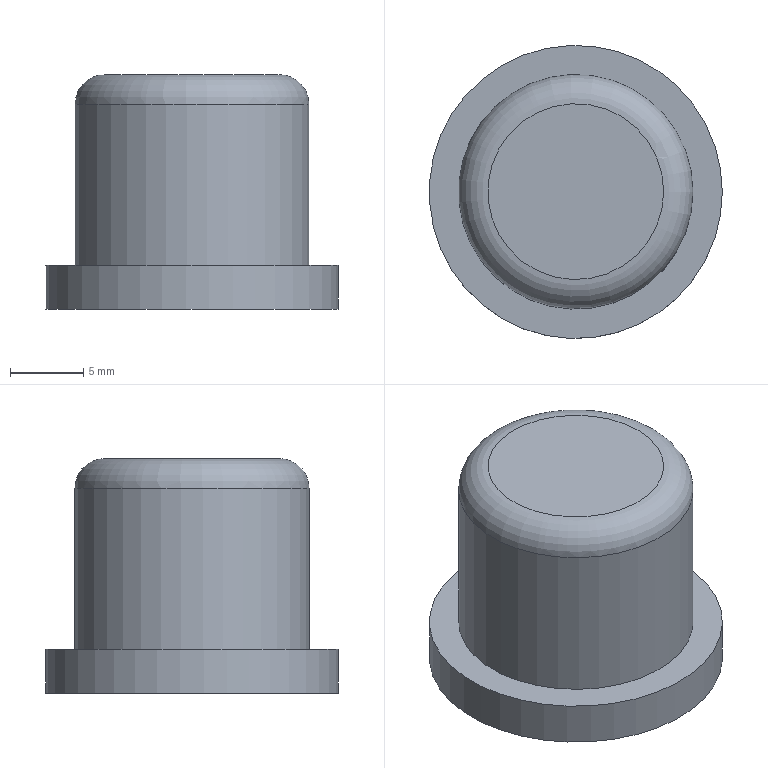Part | STEP file | 1 solid | 6 faces | box 20 x 20 x 16 mm | volume 3516 mm3 | plane 3 | cylinder 2 | torus 1 | commonest cylinder face diameters 16 x1 20 x1
STEP:
#1=CARTESIAN_POINT('',(0.,0.,0.));
#2=DIRECTION('',(0.,0.,1.));
#3=DIRECTION('',(1.,0.,0.));
#4=AXIS2_PLACEMENT_3D('',#1,#2,#3);
#5=CARTESIAN_POINT('',(1346.247,368.48,-86.181));
#6=VERTEX_POINT('',#5);
#7=CARTESIAN_POINT('',(1340.247,368.48,-86.181));
#8=DIRECTION('',(0.,0.,-1.));
#9=DIRECTION('',(1.,0.,0.));
#10=AXIS2_PLACEMENT_3D('',#7,#8,#9);
#11=CIRCLE('',#10,6.);
#12=CARTESIAN_POINT('',(1534.247,516.48,-86.181));
#13=DIRECTION('',(0.,0.,1.));
#14=DIRECTION('',(1.,0.,0.));
#15=AXIS2_PLACEMENT_3D('',#12,#13,#14);
#16=PLANE('',#15);
#17=CARTESIAN_POINT('',(-188.,-148.));
#18=CARTESIAN_POINT('',(-188.,-158.392));
#19=CARTESIAN_POINT('',(-197.,-153.196));
#20=CARTESIAN_POINT('',(-206.,-148.));
#21=CARTESIAN_POINT('',(-197.,-142.804));
#22=CARTESIAN_POINT('',(-188.,-137.608));
#23=CARTESIAN_POINT('',(-188.,-148.));
#24=(BOUNDED_CURVE()B_SPLINE_CURVE(2,(#17,#18,#19,#20,#21,#22,#23),.UNSPECIFIED.,.T.,.F.)B_SPLINE_CURVE_WITH_KNOTS((1,2,2,2,2,1),(-2.094,0.,2.094,4.189,6.283,8.378),.UNSPECIFIED.)CURVE()GEOMETRIC_REPRESENTATION_ITEM()RATIONAL_B_SPLINE_CURVE((1.,0.5,1.,0.5,1.,0.5,1.))REPRESENTATION_ITEM(''));
#25=(GEOMETRIC_REPRESENTATION_CONTEXT(2)PARAMETRIC_REPRESENTATION_CONTEXT()REPRESENTATION_CONTEXT('',''));
#26=DEFINITIONAL_REPRESENTATION('',(#24),#25);
#27=PCURVE('',#16,#26);
#28=CARTESIAN_POINT('',(1340.247,368.48,-88.181));
#29=DIRECTION('',(0.,0.,1.));
#30=DIRECTION('',(-1.,0.,0.));
#31=AXIS2_PLACEMENT_3D('',#28,#29,#30);
#32=TOROIDAL_SURFACE('',#31,6.,2.);
#33=CARTESIAN_POINT('',(9.425,7.854));
#34=DIRECTION('',(-1.,0.));
#35=VECTOR('',#34,1.);
#36=LINE('',#33,#35);
#37=(GEOMETRIC_REPRESENTATION_CONTEXT(2)PARAMETRIC_REPRESENTATION_CONTEXT()REPRESENTATION_CONTEXT('',''));
#38=DEFINITIONAL_REPRESENTATION('',(#36),#37);
#39=PCURVE('',#32,#38);
#40=SURFACE_CURVE('',#11,(#27,#39),.PCURVE_S1.);
#41=EDGE_CURVE('',#6,#6,#40,.T.);
#42=ORIENTED_EDGE('',*,*,#41,.F.);
#43=EDGE_LOOP('',(#42));
#44=FACE_BOUND('',#43,.T.);
#45=ADVANCED_FACE('',(#44),#16,.T.);
#46=CARTESIAN_POINT('',(1350.247,368.48,-102.181));
#47=VERTEX_POINT('',#46);
#48=CARTESIAN_POINT('',(1340.247,368.48,-102.181));
#49=DIRECTION('',(0.,0.,1.));
#50=DIRECTION('',(1.,0.,0.));
#51=AXIS2_PLACEMENT_3D('',#48,#49,#50);
#52=CIRCLE('',#51,10.);
#53=CARTESIAN_POINT('',(1340.247,368.48,-102.181));
#54=DIRECTION('',(0.,0.,1.));
#55=DIRECTION('',(-1.,0.,0.));
#56=AXIS2_PLACEMENT_3D('',#53,#54,#55);
#57=PLANE('',#56);
#58=CARTESIAN_POINT('',(0.,0.));
#59=DIRECTION('',(-1.,0.));
#60=AXIS2_PLACEMENT_2D('',#58,#59);
#61=CIRCLE('',#60,10.);
#62=(GEOMETRIC_REPRESENTATION_CONTEXT(2)PARAMETRIC_REPRESENTATION_CONTEXT()REPRESENTATION_CONTEXT('',''));
#63=DEFINITIONAL_REPRESENTATION('',(#61),#62);
#64=PCURVE('',#57,#63);
#65=CARTESIAN_POINT('',(1340.247,368.48,-99.181));
#66=DIRECTION('',(0.,0.,-1.));
#67=DIRECTION('',(1.,0.,0.));
#68=AXIS2_PLACEMENT_3D('',#65,#66,#67);
#69=CYLINDRICAL_SURFACE('',#68,10.);
#70=CARTESIAN_POINT('',(6.283,3.));
#71=DIRECTION('',(-1.,0.));
#72=VECTOR('',#71,1.);
#73=LINE('',#70,#72);
#74=(GEOMETRIC_REPRESENTATION_CONTEXT(2)PARAMETRIC_REPRESENTATION_CONTEXT()REPRESENTATION_CONTEXT('',''));
#75=DEFINITIONAL_REPRESENTATION('',(#73),#74);
#76=PCURVE('',#69,#75);
#77=SURFACE_CURVE('',#52,(#64,#76),.PCURVE_S1.);
#78=EDGE_CURVE('',#47,#47,#77,.T.);
#79=ORIENTED_EDGE('',*,*,#78,.F.);
#80=EDGE_LOOP('',(#79));
#81=FACE_BOUND('',#80,.T.);
#82=ADVANCED_FACE('',(#81),#57,.F.);
#83=CARTESIAN_POINT('',(1350.247,368.48,-99.181));
#84=VERTEX_POINT('',#83);
#85=CARTESIAN_POINT('',(1340.247,368.48,-99.181));
#86=DIRECTION('',(0.,0.,1.));
#87=DIRECTION('',(1.,0.,0.));
#88=AXIS2_PLACEMENT_3D('',#85,#86,#87);
#89=CIRCLE('',#88,10.);
#90=CARTESIAN_POINT('',(6.283,0.));
#91=DIRECTION('',(-1.,0.));
#92=VECTOR('',#91,1.);
#93=LINE('',#90,#92);
#94=(GEOMETRIC_REPRESENTATION_CONTEXT(2)PARAMETRIC_REPRESENTATION_CONTEXT()REPRESENTATION_CONTEXT('',''));
#95=DEFINITIONAL_REPRESENTATION('',(#93),#94);
#96=PCURVE('',#69,#95);
#97=CARTESIAN_POINT('',(1340.247,368.48,-99.181));
#98=DIRECTION('',(0.,0.,1.));
#99=DIRECTION('',(-1.,0.,0.));
#100=AXIS2_PLACEMENT_3D('',#97,#98,#99);
#101=PLANE('',#100);
#102=CARTESIAN_POINT('',(0.,0.));
#103=DIRECTION('',(-1.,0.));
#104=AXIS2_PLACEMENT_2D('',#102,#103);
#105=CIRCLE('',#104,10.);
#106=(GEOMETRIC_REPRESENTATION_CONTEXT(2)PARAMETRIC_REPRESENTATION_CONTEXT()REPRESENTATION_CONTEXT('',''));
#107=DEFINITIONAL_REPRESENTATION('',(#105),#106);
#108=PCURVE('',#101,#107);
#109=SURFACE_CURVE('',#89,(#96,#108),.PCURVE_S1.);
#110=EDGE_CURVE('',#84,#84,#109,.T.);
#111=ORIENTED_EDGE('',*,*,#110,.F.);
#112=CARTESIAN_POINT('',(1350.247,368.48,-99.181));
#113=CARTESIAN_POINT('',(1350.247,368.48,-102.181));
#114=B_SPLINE_CURVE_WITH_KNOTS('',1,(#112,#113),.UNSPECIFIED.,.F.,.F.,(2,2),(0.,3.),.PIECEWISE_BEZIER_KNOTS.);
#115=CARTESIAN_POINT('',(6.283,0.));
#116=DIRECTION('',(0.,1.));
#117=VECTOR('',#116,1.);
#118=LINE('',#115,#117);
#119=(GEOMETRIC_REPRESENTATION_CONTEXT(2)PARAMETRIC_REPRESENTATION_CONTEXT()REPRESENTATION_CONTEXT('',''));
#120=DEFINITIONAL_REPRESENTATION('',(#118),#119);
#121=PCURVE('',#69,#120);
#122=CARTESIAN_POINT('',(0.,0.));
#123=DIRECTION('',(0.,1.));
#124=VECTOR('',#123,1.);
#125=LINE('',#122,#124);
#126=(GEOMETRIC_REPRESENTATION_CONTEXT(2)PARAMETRIC_REPRESENTATION_CONTEXT()REPRESENTATION_CONTEXT('',''));
#127=DEFINITIONAL_REPRESENTATION('',(#125),#126);
#128=PCURVE('',#69,#127);
#129=SEAM_CURVE('',#114,(#121,#128),.PCURVE_S1.);
#130=EDGE_CURVE('',#84,#47,#129,.T.);
#131=ORIENTED_EDGE('',*,*,#130,.T.);
#132=ORIENTED_EDGE('',*,*,#78,.T.);
#133=ORIENTED_EDGE('',*,*,#130,.F.);
#134=EDGE_LOOP('',(#111,#131,#132,#133));
#135=FACE_BOUND('',#134,.T.);
#136=ADVANCED_FACE('',(#135),#69,.T.);
#137=CARTESIAN_POINT('',(1348.247,368.48,-99.181));
#138=VERTEX_POINT('',#137);
#139=CARTESIAN_POINT('',(1340.247,368.48,-99.181));
#140=DIRECTION('',(0.,0.,1.));
#141=DIRECTION('',(1.,0.,0.));
#142=AXIS2_PLACEMENT_3D('',#139,#140,#141);
#143=CIRCLE('',#142,8.);
#144=CARTESIAN_POINT('',(0.,0.));
#145=DIRECTION('',(-1.,0.));
#146=AXIS2_PLACEMENT_2D('',#144,#145);
#147=CIRCLE('',#146,8.);
#148=(GEOMETRIC_REPRESENTATION_CONTEXT(2)PARAMETRIC_REPRESENTATION_CONTEXT()REPRESENTATION_CONTEXT('',''));
#149=DEFINITIONAL_REPRESENTATION('',(#147),#148);
#150=PCURVE('',#101,#149);
#151=CARTESIAN_POINT('',(1340.247,368.48,-71.781));
#152=DIRECTION('',(0.,0.,-1.));
#153=DIRECTION('',(1.,0.,0.));
#154=AXIS2_PLACEMENT_3D('',#151,#152,#153);
#155=CYLINDRICAL_SURFACE('',#154,8.);
#156=CARTESIAN_POINT('',(6.283,27.4));
#157=DIRECTION('',(-1.,0.));
#158=VECTOR('',#157,1.);
#159=LINE('',#156,#158);
#160=(GEOMETRIC_REPRESENTATION_CONTEXT(2)PARAMETRIC_REPRESENTATION_CONTEXT()REPRESENTATION_CONTEXT('',''));
#161=DEFINITIONAL_REPRESENTATION('',(#159),#160);
#162=PCURVE('',#155,#161);
#163=SURFACE_CURVE('',#143,(#150,#162),.PCURVE_S1.);
#164=EDGE_CURVE('',#138,#138,#163,.T.);
#165=ORIENTED_EDGE('',*,*,#164,.F.);
#166=EDGE_LOOP('',(#165));
#167=FACE_BOUND('',#166,.T.);
#168=ORIENTED_EDGE('',*,*,#110,.T.);
#169=EDGE_LOOP('',(#168));
#170=FACE_BOUND('',#169,.T.);
#171=ADVANCED_FACE('',(#167,#170),#101,.T.);
#172=CARTESIAN_POINT('',(1348.247,368.48,-88.181));
#173=VERTEX_POINT('',#172);
#174=CARTESIAN_POINT('',(1340.247,368.48,-88.181));
#175=DIRECTION('',(0.,0.,-1.));
#176=DIRECTION('',(1.,0.,0.));
#177=AXIS2_PLACEMENT_3D('',#174,#175,#176);
#178=CIRCLE('',#177,8.);
#179=CARTESIAN_POINT('',(0.,16.4));
#180=DIRECTION('',(1.,0.));
#181=VECTOR('',#180,1.);
#182=LINE('',#179,#181);
#183=(GEOMETRIC_REPRESENTATION_CONTEXT(2)PARAMETRIC_REPRESENTATION_CONTEXT()REPRESENTATION_CONTEXT('',''));
#184=DEFINITIONAL_REPRESENTATION('',(#182),#183);
#185=PCURVE('',#155,#184);
#186=CARTESIAN_POINT('',(9.425,6.283));
#187=DIRECTION('',(-1.,0.));
#188=VECTOR('',#187,1.);
#189=LINE('',#186,#188);
#190=(GEOMETRIC_REPRESENTATION_CONTEXT(2)PARAMETRIC_REPRESENTATION_CONTEXT()REPRESENTATION_CONTEXT('',''));
#191=DEFINITIONAL_REPRESENTATION('',(#189),#190);
#192=PCURVE('',#32,#191);
#193=SURFACE_CURVE('',#178,(#185,#192),.PCURVE_S1.);
#194=EDGE_CURVE('',#173,#173,#193,.T.);
#195=ORIENTED_EDGE('',*,*,#194,.T.);
#196=CARTESIAN_POINT('',(1348.247,368.48,-88.181));
#197=CARTESIAN_POINT('',(1348.247,368.48,-99.181));
#198=B_SPLINE_CURVE_WITH_KNOTS('',1,(#196,#197),.UNSPECIFIED.,.F.,.F.,(2,2),(16.4,27.4),.PIECEWISE_BEZIER_KNOTS.);
#199=CARTESIAN_POINT('',(6.283,0.));
#200=DIRECTION('',(0.,1.));
#201=VECTOR('',#200,1.);
#202=LINE('',#199,#201);
#203=(GEOMETRIC_REPRESENTATION_CONTEXT(2)PARAMETRIC_REPRESENTATION_CONTEXT()REPRESENTATION_CONTEXT('',''));
#204=DEFINITIONAL_REPRESENTATION('',(#202),#203);
#205=PCURVE('',#155,#204);
#206=CARTESIAN_POINT('',(0.,0.));
#207=DIRECTION('',(0.,1.));
#208=VECTOR('',#207,1.);
#209=LINE('',#206,#208);
#210=(GEOMETRIC_REPRESENTATION_CONTEXT(2)PARAMETRIC_REPRESENTATION_CONTEXT()REPRESENTATION_CONTEXT('',''));
#211=DEFINITIONAL_REPRESENTATION('',(#209),#210);
#212=PCURVE('',#155,#211);
#213=SEAM_CURVE('',#198,(#205,#212),.PCURVE_S1.);
#214=EDGE_CURVE('',#173,#138,#213,.T.);
#215=ORIENTED_EDGE('',*,*,#214,.T.);
#216=ORIENTED_EDGE('',*,*,#164,.T.);
#217=ORIENTED_EDGE('',*,*,#214,.F.);
#218=EDGE_LOOP('',(#195,#215,#216,#217));
#219=FACE_BOUND('',#218,.T.);
#220=ADVANCED_FACE('',(#219),#155,.T.);
#221=ORIENTED_EDGE('',*,*,#194,.F.);
#222=CARTESIAN_POINT('',(1348.247,368.48,-88.181));
#223=CARTESIAN_POINT('',(1348.247,368.48,-87.646));
#224=CARTESIAN_POINT('',(1348.077,368.48,-87.126));
#225=CARTESIAN_POINT('',(1347.751,368.48,-86.677));
#226=CARTESIAN_POINT('',(1347.303,368.48,-86.351));
#227=CARTESIAN_POINT('',(1346.782,368.48,-86.181));
#228=CARTESIAN_POINT('',(1346.247,368.48,-86.181));
#229=(BOUNDED_CURVE()B_SPLINE_CURVE(6,(#222,#223,#224,#225,#226,#227,#228),.UNSPECIFIED.,.F.,.F.)B_SPLINE_CURVE_WITH_KNOTS((7,7),(0.,1.571),.PIECEWISE_BEZIER_KNOTS.)CURVE()GEOMETRIC_REPRESENTATION_ITEM()RATIONAL_B_SPLINE_CURVE((1.031,1.01,0.9979,0.994,0.9979,1.01,1.031))REPRESENTATION_ITEM(''));
#230=CARTESIAN_POINT('',(9.425,6.283));
#231=DIRECTION('',(0.,1.));
#232=VECTOR('',#231,1.);
#233=LINE('',#230,#232);
#234=(GEOMETRIC_REPRESENTATION_CONTEXT(2)PARAMETRIC_REPRESENTATION_CONTEXT()REPRESENTATION_CONTEXT('',''));
#235=DEFINITIONAL_REPRESENTATION('',(#233),#234);
#236=PCURVE('',#32,#235);
#237=CARTESIAN_POINT('',(3.142,6.283));
#238=DIRECTION('',(0.,1.));
#239=VECTOR('',#238,1.);
#240=LINE('',#237,#239);
#241=(GEOMETRIC_REPRESENTATION_CONTEXT(2)PARAMETRIC_REPRESENTATION_CONTEXT()REPRESENTATION_CONTEXT('',''));
#242=DEFINITIONAL_REPRESENTATION('',(#240),#241);
#243=PCURVE('',#32,#242);
#244=SEAM_CURVE('',#229,(#236,#243),.PCURVE_S1.);
#245=EDGE_CURVE('',#173,#6,#244,.T.);
#246=ORIENTED_EDGE('',*,*,#245,.T.);
#247=ORIENTED_EDGE('',*,*,#41,.T.);
#248=ORIENTED_EDGE('',*,*,#245,.F.);
#249=EDGE_LOOP('',(#221,#246,#247,#248));
#250=FACE_BOUND('',#249,.T.);
#251=ADVANCED_FACE('',(#250),#32,.T.);
#252=CLOSED_SHELL('',(#45,#82,#136,#171,#220,#251));
#253=MANIFOLD_SOLID_BREP('',#252);
#254=(LENGTH_UNIT()NAMED_UNIT(*)SI_UNIT(.MILLI.,.METRE.));
#255=UNCERTAINTY_MEASURE_WITH_UNIT(LENGTH_MEASURE(0.00001),#254,'','');
#256=(NAMED_UNIT(*)PLANE_ANGLE_UNIT()SI_UNIT($,.RADIAN.));
#257=(NAMED_UNIT(*)SI_UNIT($,.STERADIAN.)SOLID_ANGLE_UNIT());
#258=(GEOMETRIC_REPRESENTATION_CONTEXT(3)GLOBAL_UNCERTAINTY_ASSIGNED_CONTEXT((#255))GLOBAL_UNIT_ASSIGNED_CONTEXT((#254,#256,#257))REPRESENTATION_CONTEXT('',''));
#259=ADVANCED_BREP_SHAPE_REPRESENTATION('',(#4,#253),#258);